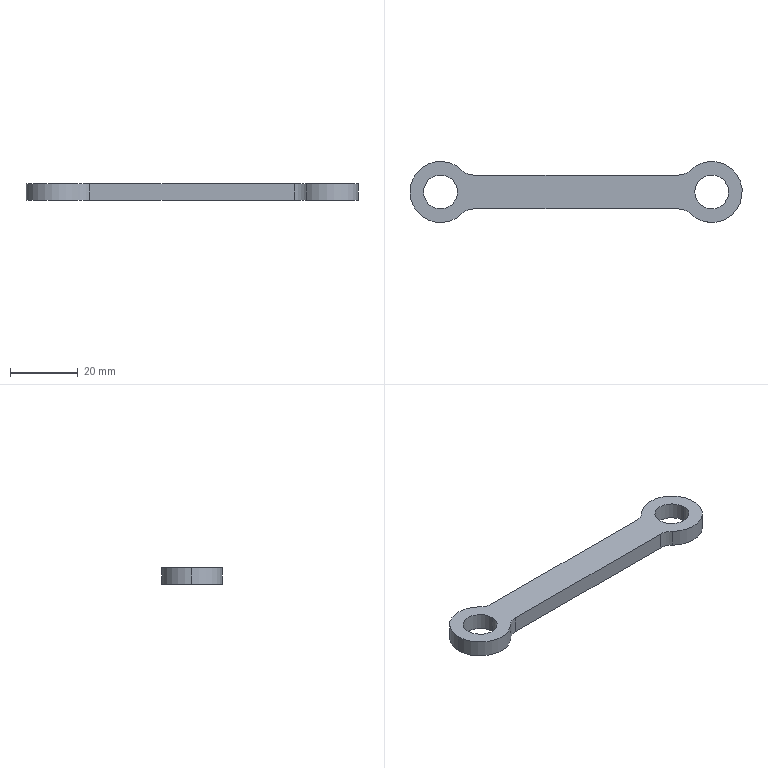Part | SolidWorks | features Extrusion 1 | 1 solid | 15 faces | box 98 x 18 x 5 mm | volume 4921 mm3 | cylinder 11 | plane 4 | commonest cylinder face diameters 10 x8 18 x3
STEP:
#1=CARTESIAN_POINT('',(75.,0.,5.));
#2=VERTEX_POINT('',#1);
#3=CARTESIAN_POINT('',(85.,0.,5.));
#4=VERTEX_POINT('',#3);
#5=CARTESIAN_POINT('',(80.,0.,5.));
#6=DIRECTION('',(0.,0.,1.));
#7=DIRECTION('',(1.,0.,0.));
#8=AXIS2_PLACEMENT_3D('',#5,#6,#7);
#9=CIRCLE('',#8,5.);
#10=EDGE_CURVE('',#2,#4,#9,.T.);
#11=ORIENTED_EDGE('',*,*,#10,.T.);
#12=CARTESIAN_POINT('',(85.,0.,0.));
#13=VERTEX_POINT('',#12);
#14=CARTESIAN_POINT('',(85.,0.,5.));
#15=DIRECTION('',(0.,0.,-1.));
#16=VECTOR('',#15,1000.);
#17=LINE('',#14,#16);
#18=EDGE_CURVE('',#4,#13,#17,.T.);
#19=ORIENTED_EDGE('',*,*,#18,.T.);
#20=CARTESIAN_POINT('',(75.,0.,0.));
#21=VERTEX_POINT('',#20);
#22=CARTESIAN_POINT('',(80.,0.,0.));
#23=DIRECTION('',(0.,0.,1.));
#24=DIRECTION('',(1.,0.,0.));
#25=AXIS2_PLACEMENT_3D('',#22,#23,#24);
#26=CIRCLE('',#25,5.);
#27=EDGE_CURVE('',#21,#13,#26,.T.);
#28=ORIENTED_EDGE('',*,*,#27,.F.);
#29=CARTESIAN_POINT('',(75.,0.,5.));
#30=DIRECTION('',(0.,0.,-1.));
#31=VECTOR('',#30,1000.);
#32=LINE('',#29,#31);
#33=EDGE_CURVE('',#2,#21,#32,.T.);
#34=ORIENTED_EDGE('',*,*,#33,.F.);
#35=EDGE_LOOP('',(#11,#19,#28,#34));
#36=FACE_OUTER_BOUND('',#35,.T.);
#37=CARTESIAN_POINT('',(80.,0.,5.));
#38=DIRECTION('',(0.,0.,-1.));
#39=DIRECTION('',(-1.,0.,0.));
#40=AXIS2_PLACEMENT_3D('',#37,#38,#39);
#41=CYLINDRICAL_SURFACE('',#40,5.);
#42=ADVANCED_FACE('',(#36),#41,.F.);
#43=CARTESIAN_POINT('',(-5.,0.,5.));
#44=VERTEX_POINT('',#43);
#45=CARTESIAN_POINT('',(5.,0.,5.));
#46=VERTEX_POINT('',#45);
#47=CARTESIAN_POINT('',(0.,0.,5.));
#48=DIRECTION('',(0.,0.,1.));
#49=DIRECTION('',(1.,0.,0.));
#50=AXIS2_PLACEMENT_3D('',#47,#48,#49);
#51=CIRCLE('',#50,5.);
#52=EDGE_CURVE('',#44,#46,#51,.T.);
#53=ORIENTED_EDGE('',*,*,#52,.T.);
#54=CARTESIAN_POINT('',(5.,0.,0.));
#55=VERTEX_POINT('',#54);
#56=CARTESIAN_POINT('',(5.,0.,5.));
#57=DIRECTION('',(0.,0.,-1.));
#58=VECTOR('',#57,1000.);
#59=LINE('',#56,#58);
#60=EDGE_CURVE('',#46,#55,#59,.T.);
#61=ORIENTED_EDGE('',*,*,#60,.T.);
#62=CARTESIAN_POINT('',(-5.,0.,0.));
#63=VERTEX_POINT('',#62);
#64=CARTESIAN_POINT('',(0.,0.,0.));
#65=DIRECTION('',(0.,0.,1.));
#66=DIRECTION('',(1.,0.,0.));
#67=AXIS2_PLACEMENT_3D('',#64,#65,#66);
#68=CIRCLE('',#67,5.);
#69=EDGE_CURVE('',#63,#55,#68,.T.);
#70=ORIENTED_EDGE('',*,*,#69,.F.);
#71=CARTESIAN_POINT('',(-5.,0.,5.));
#72=DIRECTION('',(0.,0.,-1.));
#73=VECTOR('',#72,1000.);
#74=LINE('',#71,#73);
#75=EDGE_CURVE('',#44,#63,#74,.T.);
#76=ORIENTED_EDGE('',*,*,#75,.F.);
#77=EDGE_LOOP('',(#53,#61,#70,#76));
#78=FACE_OUTER_BOUND('',#77,.T.);
#79=CARTESIAN_POINT('',(0.,0.,5.));
#80=DIRECTION('',(0.,0.,-1.));
#81=DIRECTION('',(-1.,0.,0.));
#82=AXIS2_PLACEMENT_3D('',#79,#80,#81);
#83=CYLINDRICAL_SURFACE('',#82,5.);
#84=ADVANCED_FACE('',(#78),#83,.F.);
#85=CARTESIAN_POINT('',(-9.,0.,5.));
#86=VERTEX_POINT('',#85);
#87=CARTESIAN_POINT('',(6.299,-6.429,5.));
#88=VERTEX_POINT('',#87);
#89=CARTESIAN_POINT('',(0.,0.,5.));
#90=DIRECTION('',(0.,0.,1.));
#91=DIRECTION('',(1.,0.,0.));
#92=AXIS2_PLACEMENT_3D('',#89,#90,#91);
#93=CIRCLE('',#92,9.);
#94=EDGE_CURVE('',#86,#88,#93,.T.);
#95=ORIENTED_EDGE('',*,*,#94,.F.);
#96=CARTESIAN_POINT('',(-9.,0.,0.));
#97=VERTEX_POINT('',#96);
#98=CARTESIAN_POINT('',(-9.,0.,5.));
#99=DIRECTION('',(0.,0.,-1.));
#100=VECTOR('',#99,1000.);
#101=LINE('',#98,#100);
#102=EDGE_CURVE('',#86,#97,#101,.T.);
#103=ORIENTED_EDGE('',*,*,#102,.T.);
#104=CARTESIAN_POINT('',(6.299,-6.429,0.));
#105=VERTEX_POINT('',#104);
#106=CARTESIAN_POINT('',(0.,0.,0.));
#107=DIRECTION('',(0.,0.,1.));
#108=DIRECTION('',(1.,0.,0.));
#109=AXIS2_PLACEMENT_3D('',#106,#107,#108);
#110=CIRCLE('',#109,9.);
#111=EDGE_CURVE('',#97,#105,#110,.T.);
#112=ORIENTED_EDGE('',*,*,#111,.T.);
#113=CARTESIAN_POINT('',(6.299,-6.429,5.));
#114=DIRECTION('',(0.,0.,-1.));
#115=VECTOR('',#114,1000.);
#116=LINE('',#113,#115);
#117=EDGE_CURVE('',#88,#105,#116,.T.);
#118=ORIENTED_EDGE('',*,*,#117,.F.);
#119=EDGE_LOOP('',(#95,#103,#112,#118));
#120=FACE_OUTER_BOUND('',#119,.T.);
#121=CARTESIAN_POINT('',(0.,0.,5.));
#122=DIRECTION('',(0.,0.,-1.));
#123=DIRECTION('',(-1.,0.,0.));
#124=AXIS2_PLACEMENT_3D('',#121,#122,#123);
#125=CYLINDRICAL_SURFACE('',#124,9.);
#126=ADVANCED_FACE('',(#120),#125,.T.);
#127=ORIENTED_EDGE('',*,*,#52,.F.);
#128=CARTESIAN_POINT('',(0.,0.,5.));
#129=DIRECTION('',(0.,0.,1.));
#130=DIRECTION('',(1.,0.,0.));
#131=AXIS2_PLACEMENT_3D('',#128,#129,#130);
#132=CIRCLE('',#131,5.);
#133=EDGE_CURVE('',#46,#44,#132,.T.);
#134=ORIENTED_EDGE('',*,*,#133,.F.);
#135=EDGE_LOOP('',(#127,#134));
#136=FACE_BOUND('',#135,.T.);
#137=CARTESIAN_POINT('',(73.701,6.429,5.));
#138=VERTEX_POINT('',#137);
#139=CARTESIAN_POINT('',(70.202,5.,5.));
#140=VERTEX_POINT('',#139);
#141=CARTESIAN_POINT('',(70.202,10.,5.));
#142=DIRECTION('',(0.,0.,-1.));
#143=DIRECTION('',(1.,0.,0.));
#144=AXIS2_PLACEMENT_3D('',#141,#142,#143);
#145=CIRCLE('',#144,5.);
#146=EDGE_CURVE('',#138,#140,#145,.T.);
#147=ORIENTED_EDGE('',*,*,#146,.T.);
#148=CARTESIAN_POINT('',(9.798,5.,5.));
#149=VERTEX_POINT('',#148);
#150=CARTESIAN_POINT('',(9.798,5.,5.));
#151=DIRECTION('',(-1.,0.,0.));
#152=VECTOR('',#151,1000.);
#153=LINE('',#150,#152);
#154=EDGE_CURVE('',#140,#149,#153,.T.);
#155=ORIENTED_EDGE('',*,*,#154,.T.);
#156=CARTESIAN_POINT('',(6.299,6.429,5.));
#157=VERTEX_POINT('',#156);
#158=CARTESIAN_POINT('',(9.798,10.,5.));
#159=DIRECTION('',(0.,0.,-1.));
#160=DIRECTION('',(-1.,0.,0.));
#161=AXIS2_PLACEMENT_3D('',#158,#159,#160);
#162=CIRCLE('',#161,5.);
#163=EDGE_CURVE('',#149,#157,#162,.T.);
#164=ORIENTED_EDGE('',*,*,#163,.T.);
#165=CARTESIAN_POINT('',(0.,0.,5.));
#166=DIRECTION('',(0.,0.,1.));
#167=DIRECTION('',(1.,0.,0.));
#168=AXIS2_PLACEMENT_3D('',#165,#166,#167);
#169=CIRCLE('',#168,9.);
#170=EDGE_CURVE('',#157,#86,#169,.T.);
#171=ORIENTED_EDGE('',*,*,#170,.T.);
#172=ORIENTED_EDGE('',*,*,#94,.T.);
#173=CARTESIAN_POINT('',(9.798,-5.,5.));
#174=VERTEX_POINT('',#173);
#175=CARTESIAN_POINT('',(9.798,-10.,5.));
#176=DIRECTION('',(0.,0.,-1.));
#177=DIRECTION('',(1.,0.,0.));
#178=AXIS2_PLACEMENT_3D('',#175,#176,#177);
#179=CIRCLE('',#178,5.);
#180=EDGE_CURVE('',#88,#174,#179,.T.);
#181=ORIENTED_EDGE('',*,*,#180,.T.);
#182=CARTESIAN_POINT('',(70.202,-5.,5.));
#183=VERTEX_POINT('',#182);
#184=CARTESIAN_POINT('',(9.798,-5.,5.));
#185=DIRECTION('',(1.,0.,0.));
#186=VECTOR('',#185,1000.);
#187=LINE('',#184,#186);
#188=EDGE_CURVE('',#174,#183,#187,.T.);
#189=ORIENTED_EDGE('',*,*,#188,.T.);
#190=CARTESIAN_POINT('',(73.701,-6.429,5.));
#191=VERTEX_POINT('',#190);
#192=CARTESIAN_POINT('',(70.202,-10.,5.));
#193=DIRECTION('',(0.,0.,-1.));
#194=DIRECTION('',(-1.,0.,0.));
#195=AXIS2_PLACEMENT_3D('',#192,#193,#194);
#196=CIRCLE('',#195,5.);
#197=EDGE_CURVE('',#183,#191,#196,.T.);
#198=ORIENTED_EDGE('',*,*,#197,.T.);
#199=CARTESIAN_POINT('',(80.,0.,5.));
#200=DIRECTION('',(0.,0.,1.));
#201=DIRECTION('',(1.,0.,0.));
#202=AXIS2_PLACEMENT_3D('',#199,#200,#201);
#203=CIRCLE('',#202,9.);
#204=EDGE_CURVE('',#191,#138,#203,.T.);
#205=ORIENTED_EDGE('',*,*,#204,.T.);
#206=EDGE_LOOP('',(#147,#155,#164,#171,#172,#181,#189,#198,#205));
#207=FACE_OUTER_BOUND('',#206,.T.);
#208=ORIENTED_EDGE('',*,*,#10,.F.);
#209=CARTESIAN_POINT('',(80.,0.,5.));
#210=DIRECTION('',(0.,0.,1.));
#211=DIRECTION('',(1.,0.,0.));
#212=AXIS2_PLACEMENT_3D('',#209,#210,#211);
#213=CIRCLE('',#212,5.);
#214=EDGE_CURVE('',#4,#2,#213,.T.);
#215=ORIENTED_EDGE('',*,*,#214,.F.);
#216=EDGE_LOOP('',(#208,#215));
#217=FACE_BOUND('',#216,.T.);
#218=CARTESIAN_POINT('',(70.202,10.,5.));
#219=DIRECTION('',(0.,0.,1.));
#220=DIRECTION('',(1.,0.,0.));
#221=AXIS2_PLACEMENT_3D('',#218,#219,#220);
#222=PLANE('',#221);
#223=ADVANCED_FACE('',(#136,#207,#217),#222,.T.);
#224=CARTESIAN_POINT('',(73.701,6.429,0.));
#225=VERTEX_POINT('',#224);
#226=CARTESIAN_POINT('',(70.202,5.,0.));
#227=VERTEX_POINT('',#226);
#228=CARTESIAN_POINT('',(70.202,10.,0.));
#229=DIRECTION('',(0.,0.,-1.));
#230=DIRECTION('',(1.,0.,0.));
#231=AXIS2_PLACEMENT_3D('',#228,#229,#230);
#232=CIRCLE('',#231,5.);
#233=EDGE_CURVE('',#225,#227,#232,.T.);
#234=ORIENTED_EDGE('',*,*,#233,.F.);
#235=CARTESIAN_POINT('',(73.701,-6.429,0.));
#236=VERTEX_POINT('',#235);
#237=CARTESIAN_POINT('',(80.,0.,0.));
#238=DIRECTION('',(0.,0.,1.));
#239=DIRECTION('',(1.,0.,0.));
#240=AXIS2_PLACEMENT_3D('',#237,#238,#239);
#241=CIRCLE('',#240,9.);
#242=EDGE_CURVE('',#236,#225,#241,.T.);
#243=ORIENTED_EDGE('',*,*,#242,.F.);
#244=CARTESIAN_POINT('',(70.202,-5.,0.));
#245=VERTEX_POINT('',#244);
#246=CARTESIAN_POINT('',(70.202,-10.,0.));
#247=DIRECTION('',(0.,0.,-1.));
#248=DIRECTION('',(-1.,0.,0.));
#249=AXIS2_PLACEMENT_3D('',#246,#247,#248);
#250=CIRCLE('',#249,5.);
#251=EDGE_CURVE('',#245,#236,#250,.T.);
#252=ORIENTED_EDGE('',*,*,#251,.F.);
#253=CARTESIAN_POINT('',(9.798,-5.,0.));
#254=VERTEX_POINT('',#253);
#255=CARTESIAN_POINT('',(9.798,-5.,0.));
#256=DIRECTION('',(1.,0.,0.));
#257=VECTOR('',#256,1000.);
#258=LINE('',#255,#257);
#259=EDGE_CURVE('',#254,#245,#258,.T.);
#260=ORIENTED_EDGE('',*,*,#259,.F.);
#261=CARTESIAN_POINT('',(9.798,-10.,0.));
#262=DIRECTION('',(0.,0.,-1.));
#263=DIRECTION('',(1.,0.,0.));
#264=AXIS2_PLACEMENT_3D('',#261,#262,#263);
#265=CIRCLE('',#264,5.);
#266=EDGE_CURVE('',#105,#254,#265,.T.);
#267=ORIENTED_EDGE('',*,*,#266,.F.);
#268=ORIENTED_EDGE('',*,*,#111,.F.);
#269=CARTESIAN_POINT('',(6.299,6.429,0.));
#270=VERTEX_POINT('',#269);
#271=CARTESIAN_POINT('',(0.,0.,0.));
#272=DIRECTION('',(0.,0.,1.));
#273=DIRECTION('',(1.,0.,0.));
#274=AXIS2_PLACEMENT_3D('',#271,#272,#273);
#275=CIRCLE('',#274,9.);
#276=EDGE_CURVE('',#270,#97,#275,.T.);
#277=ORIENTED_EDGE('',*,*,#276,.F.);
#278=CARTESIAN_POINT('',(9.798,5.,0.));
#279=VERTEX_POINT('',#278);
#280=CARTESIAN_POINT('',(9.798,10.,0.));
#281=DIRECTION('',(0.,0.,-1.));
#282=DIRECTION('',(-1.,0.,0.));
#283=AXIS2_PLACEMENT_3D('',#280,#281,#282);
#284=CIRCLE('',#283,5.);
#285=EDGE_CURVE('',#279,#270,#284,.T.);
#286=ORIENTED_EDGE('',*,*,#285,.F.);
#287=CARTESIAN_POINT('',(9.798,5.,0.));
#288=DIRECTION('',(-1.,0.,0.));
#289=VECTOR('',#288,1000.);
#290=LINE('',#287,#289);
#291=EDGE_CURVE('',#227,#279,#290,.T.);
#292=ORIENTED_EDGE('',*,*,#291,.F.);
#293=EDGE_LOOP('',(#234,#243,#252,#260,#267,#268,#277,#286,#292));
#294=FACE_OUTER_BOUND('',#293,.T.);
#295=ORIENTED_EDGE('',*,*,#69,.T.);
#296=CARTESIAN_POINT('',(0.,0.,0.));
#297=DIRECTION('',(0.,0.,1.));
#298=DIRECTION('',(1.,0.,0.));
#299=AXIS2_PLACEMENT_3D('',#296,#297,#298);
#300=CIRCLE('',#299,5.);
#301=EDGE_CURVE('',#55,#63,#300,.T.);
#302=ORIENTED_EDGE('',*,*,#301,.T.);
#303=EDGE_LOOP('',(#295,#302));
#304=FACE_BOUND('',#303,.T.);
#305=ORIENTED_EDGE('',*,*,#27,.T.);
#306=CARTESIAN_POINT('',(80.,0.,0.));
#307=DIRECTION('',(0.,0.,1.));
#308=DIRECTION('',(1.,0.,0.));
#309=AXIS2_PLACEMENT_3D('',#306,#307,#308);
#310=CIRCLE('',#309,5.);
#311=EDGE_CURVE('',#13,#21,#310,.T.);
#312=ORIENTED_EDGE('',*,*,#311,.T.);
#313=EDGE_LOOP('',(#305,#312));
#314=FACE_BOUND('',#313,.T.);
#315=CARTESIAN_POINT('',(70.202,10.,0.));
#316=DIRECTION('',(0.,0.,1.));
#317=DIRECTION('',(1.,0.,0.));
#318=AXIS2_PLACEMENT_3D('',#315,#316,#317);
#319=PLANE('',#318);
#320=ADVANCED_FACE('',(#294,#304,#314),#319,.F.);
#321=ORIENTED_EDGE('',*,*,#233,.T.);
#322=CARTESIAN_POINT('',(70.202,5.,5.));
#323=DIRECTION('',(0.,0.,-1.));
#324=VECTOR('',#323,1000.);
#325=LINE('',#322,#324);
#326=EDGE_CURVE('',#140,#227,#325,.T.);
#327=ORIENTED_EDGE('',*,*,#326,.F.);
#328=ORIENTED_EDGE('',*,*,#146,.F.);
#329=CARTESIAN_POINT('',(73.701,6.429,5.));
#330=DIRECTION('',(0.,0.,-1.));
#331=VECTOR('',#330,1000.);
#332=LINE('',#329,#331);
#333=EDGE_CURVE('',#138,#225,#332,.T.);
#334=ORIENTED_EDGE('',*,*,#333,.T.);
#335=EDGE_LOOP('',(#321,#327,#328,#334));
#336=FACE_OUTER_BOUND('',#335,.T.);
#337=CARTESIAN_POINT('',(70.202,10.,5.));
#338=DIRECTION('',(0.,0.,-1.));
#339=DIRECTION('',(-1.,0.,0.));
#340=AXIS2_PLACEMENT_3D('',#337,#338,#339);
#341=CYLINDRICAL_SURFACE('',#340,5.);
#342=ADVANCED_FACE('',(#336),#341,.F.);
#343=ORIENTED_EDGE('',*,*,#291,.T.);
#344=CARTESIAN_POINT('',(9.798,5.,5.));
#345=DIRECTION('',(0.,0.,-1.));
#346=VECTOR('',#345,1000.);
#347=LINE('',#344,#346);
#348=EDGE_CURVE('',#149,#279,#347,.T.);
#349=ORIENTED_EDGE('',*,*,#348,.F.);
#350=ORIENTED_EDGE('',*,*,#154,.F.);
#351=ORIENTED_EDGE('',*,*,#326,.T.);
#352=EDGE_LOOP('',(#343,#349,#350,#351));
#353=FACE_OUTER_BOUND('',#352,.T.);
#354=CARTESIAN_POINT('',(9.798,5.,5.));
#355=DIRECTION('',(0.,-1.,0.));
#356=DIRECTION('',(0.,0.,-1.));
#357=AXIS2_PLACEMENT_3D('',#354,#355,#356);
#358=PLANE('',#357);
#359=ADVANCED_FACE('',(#353),#358,.F.);
#360=ORIENTED_EDGE('',*,*,#285,.T.);
#361=CARTESIAN_POINT('',(6.299,6.429,5.));
#362=DIRECTION('',(0.,0.,-1.));
#363=VECTOR('',#362,1000.);
#364=LINE('',#361,#363);
#365=EDGE_CURVE('',#157,#270,#364,.T.);
#366=ORIENTED_EDGE('',*,*,#365,.F.);
#367=ORIENTED_EDGE('',*,*,#163,.F.);
#368=ORIENTED_EDGE('',*,*,#348,.T.);
#369=EDGE_LOOP('',(#360,#366,#367,#368));
#370=FACE_OUTER_BOUND('',#369,.T.);
#371=CARTESIAN_POINT('',(9.798,10.,5.));
#372=DIRECTION('',(0.,0.,-1.));
#373=DIRECTION('',(-1.,0.,0.));
#374=AXIS2_PLACEMENT_3D('',#371,#372,#373);
#375=CYLINDRICAL_SURFACE('',#374,5.);
#376=ADVANCED_FACE('',(#370),#375,.F.);
#377=ORIENTED_EDGE('',*,*,#102,.F.);
#378=ORIENTED_EDGE('',*,*,#170,.F.);
#379=ORIENTED_EDGE('',*,*,#365,.T.);
#380=ORIENTED_EDGE('',*,*,#276,.T.);
#381=EDGE_LOOP('',(#377,#378,#379,#380));
#382=FACE_OUTER_BOUND('',#381,.T.);
#383=CARTESIAN_POINT('',(0.,0.,5.));
#384=DIRECTION('',(0.,0.,-1.));
#385=DIRECTION('',(-1.,0.,0.));
#386=AXIS2_PLACEMENT_3D('',#383,#384,#385);
#387=CYLINDRICAL_SURFACE('',#386,9.);
#388=ADVANCED_FACE('',(#382),#387,.T.);
#389=ORIENTED_EDGE('',*,*,#266,.T.);
#390=CARTESIAN_POINT('',(9.798,-5.,5.));
#391=DIRECTION('',(0.,0.,-1.));
#392=VECTOR('',#391,1000.);
#393=LINE('',#390,#392);
#394=EDGE_CURVE('',#174,#254,#393,.T.);
#395=ORIENTED_EDGE('',*,*,#394,.F.);
#396=ORIENTED_EDGE('',*,*,#180,.F.);
#397=ORIENTED_EDGE('',*,*,#117,.T.);
#398=EDGE_LOOP('',(#389,#395,#396,#397));
#399=FACE_OUTER_BOUND('',#398,.T.);
#400=CARTESIAN_POINT('',(9.798,-10.,5.));
#401=DIRECTION('',(0.,0.,-1.));
#402=DIRECTION('',(-1.,0.,0.));
#403=AXIS2_PLACEMENT_3D('',#400,#401,#402);
#404=CYLINDRICAL_SURFACE('',#403,5.);
#405=ADVANCED_FACE('',(#399),#404,.F.);
#406=ORIENTED_EDGE('',*,*,#259,.T.);
#407=CARTESIAN_POINT('',(70.202,-5.,5.));
#408=DIRECTION('',(0.,0.,-1.));
#409=VECTOR('',#408,1000.);
#410=LINE('',#407,#409);
#411=EDGE_CURVE('',#183,#245,#410,.T.);
#412=ORIENTED_EDGE('',*,*,#411,.F.);
#413=ORIENTED_EDGE('',*,*,#188,.F.);
#414=ORIENTED_EDGE('',*,*,#394,.T.);
#415=EDGE_LOOP('',(#406,#412,#413,#414));
#416=FACE_OUTER_BOUND('',#415,.T.);
#417=CARTESIAN_POINT('',(9.798,-5.,5.));
#418=DIRECTION('',(0.,1.,0.));
#419=DIRECTION('',(0.,0.,1.));
#420=AXIS2_PLACEMENT_3D('',#417,#418,#419);
#421=PLANE('',#420);
#422=ADVANCED_FACE('',(#416),#421,.F.);
#423=ORIENTED_EDGE('',*,*,#251,.T.);
#424=CARTESIAN_POINT('',(73.701,-6.429,5.));
#425=DIRECTION('',(0.,0.,-1.));
#426=VECTOR('',#425,1000.);
#427=LINE('',#424,#426);
#428=EDGE_CURVE('',#191,#236,#427,.T.);
#429=ORIENTED_EDGE('',*,*,#428,.F.);
#430=ORIENTED_EDGE('',*,*,#197,.F.);
#431=ORIENTED_EDGE('',*,*,#411,.T.);
#432=EDGE_LOOP('',(#423,#429,#430,#431));
#433=FACE_OUTER_BOUND('',#432,.T.);
#434=CARTESIAN_POINT('',(70.202,-10.,5.));
#435=DIRECTION('',(0.,0.,-1.));
#436=DIRECTION('',(-1.,0.,0.));
#437=AXIS2_PLACEMENT_3D('',#434,#435,#436);
#438=CYLINDRICAL_SURFACE('',#437,5.);
#439=ADVANCED_FACE('',(#433),#438,.F.);
#440=ORIENTED_EDGE('',*,*,#242,.T.);
#441=ORIENTED_EDGE('',*,*,#333,.F.);
#442=ORIENTED_EDGE('',*,*,#204,.F.);
#443=ORIENTED_EDGE('',*,*,#428,.T.);
#444=EDGE_LOOP('',(#440,#441,#442,#443));
#445=FACE_OUTER_BOUND('',#444,.T.);
#446=CARTESIAN_POINT('',(80.,0.,5.));
#447=DIRECTION('',(0.,0.,-1.));
#448=DIRECTION('',(-1.,0.,0.));
#449=AXIS2_PLACEMENT_3D('',#446,#447,#448);
#450=CYLINDRICAL_SURFACE('',#449,9.);
#451=ADVANCED_FACE('',(#445),#450,.T.);
#452=ORIENTED_EDGE('',*,*,#60,.F.);
#453=ORIENTED_EDGE('',*,*,#133,.T.);
#454=ORIENTED_EDGE('',*,*,#75,.T.);
#455=ORIENTED_EDGE('',*,*,#301,.F.);
#456=EDGE_LOOP('',(#452,#453,#454,#455));
#457=FACE_OUTER_BOUND('',#456,.T.);
#458=CARTESIAN_POINT('',(0.,0.,5.));
#459=DIRECTION('',(0.,0.,-1.));
#460=DIRECTION('',(-1.,0.,0.));
#461=AXIS2_PLACEMENT_3D('',#458,#459,#460);
#462=CYLINDRICAL_SURFACE('',#461,5.);
#463=ADVANCED_FACE('',(#457),#462,.F.);
#464=ORIENTED_EDGE('',*,*,#18,.F.);
#465=ORIENTED_EDGE('',*,*,#214,.T.);
#466=ORIENTED_EDGE('',*,*,#33,.T.);
#467=ORIENTED_EDGE('',*,*,#311,.F.);
#468=EDGE_LOOP('',(#464,#465,#466,#467));
#469=FACE_OUTER_BOUND('',#468,.T.);
#470=CARTESIAN_POINT('',(80.,0.,5.));
#471=DIRECTION('',(0.,0.,-1.));
#472=DIRECTION('',(-1.,0.,0.));
#473=AXIS2_PLACEMENT_3D('',#470,#471,#472);
#474=CYLINDRICAL_SURFACE('',#473,5.);
#475=ADVANCED_FACE('',(#469),#474,.F.);
#476=CLOSED_SHELL('',(#42,#84,#126,#223,#320,#342,#359,#376,#388,#405,#422,#439,#451,#463,#475));
#477=MANIFOLD_SOLID_BREP('',#476);
#478=CARTESIAN_POINT('',(0.,0.,0.));
#479=DIRECTION('',(0.,0.,1.));
#480=DIRECTION('',(1.,0.,0.));
#481=AXIS2_PLACEMENT_3D('',#478,#479,#480);
#482=(LENGTH_UNIT()NAMED_UNIT(*)SI_UNIT(.MILLI.,.METRE.));
#483=UNCERTAINTY_MEASURE_WITH_UNIT(LENGTH_MEASURE(0.00001),#482,'','');
#484=(NAMED_UNIT(*)PLANE_ANGLE_UNIT()SI_UNIT($,.RADIAN.));
#485=(NAMED_UNIT(*)SI_UNIT($,.STERADIAN.)SOLID_ANGLE_UNIT());
#486=(GEOMETRIC_REPRESENTATION_CONTEXT(3)GLOBAL_UNCERTAINTY_ASSIGNED_CONTEXT((#483))GLOBAL_UNIT_ASSIGNED_CONTEXT((#482,#484,#485))REPRESENTATION_CONTEXT('',''));
#487=ADVANCED_BREP_SHAPE_REPRESENTATION('',(#477,#481),#486);